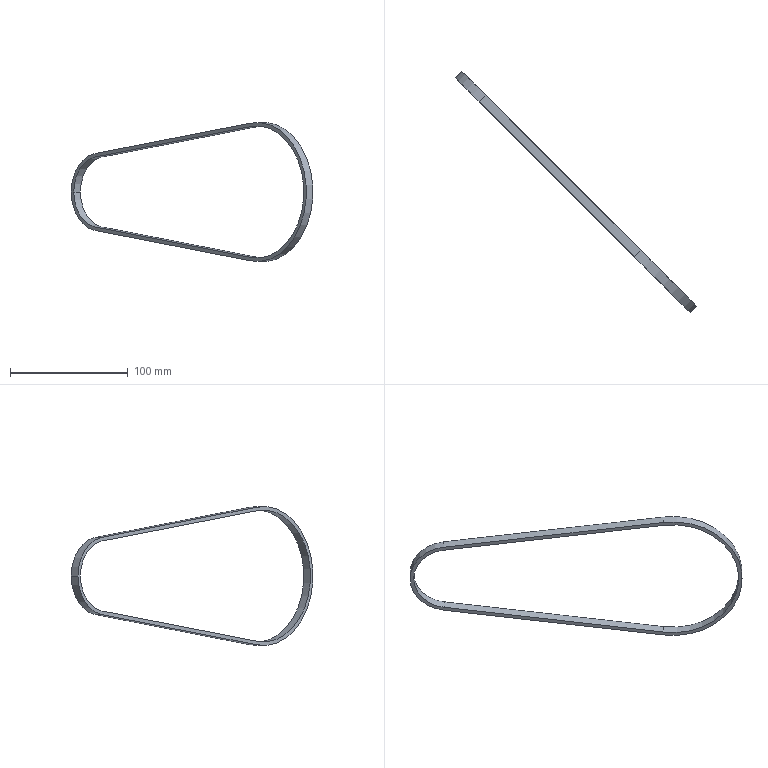Part | SolidWorks | 1 solid | 12 faces | box 205.061 x 205.061 x 118 mm | volume 15916 mm3 | cylinder 6 | plane 6 | commonest cylinder face diameters 60 x2 66 x2 112 x1 118 x1
STEP:
#1=CARTESIAN_POINT('',(92.408,296.784,-1142.11));
#2=VERTEX_POINT('',#1);
#3=CARTESIAN_POINT('',(72.266,316.925,-1109.42));
#4=VERTEX_POINT('',#3);
#5=CARTESIAN_POINT('',(95.601,293.591,-1109.42));
#6=DIRECTION('',(0.7071,0.7071,0.));
#7=DIRECTION('',(-0.7071,0.7071,0.));
#8=AXIS2_PLACEMENT_3D('',#5,#6,#7);
#9=CIRCLE('',#8,33.);
#10=EDGE_CURVE('',#2,#4,#9,.T.);
#11=ORIENTED_EDGE('',*,*,#10,.T.);
#12=CARTESIAN_POINT('',(77.923,322.582,-1109.42));
#13=VERTEX_POINT('',#12);
#14=CARTESIAN_POINT('',(77.923,322.582,-1109.42));
#15=DIRECTION('',(0.7071,0.7071,0.));
#16=VECTOR('',#15,1000.);
#17=LINE('',#14,#16);
#18=EDGE_CURVE('',#4,#13,#17,.T.);
#19=ORIENTED_EDGE('',*,*,#18,.T.);
#20=CARTESIAN_POINT('',(98.065,302.441,-1142.11));
#21=VERTEX_POINT('',#20);
#22=CARTESIAN_POINT('',(101.258,299.248,-1109.42));
#23=DIRECTION('',(-0.7071,-0.7071,0.));
#24=DIRECTION('',(-0.09676,0.09676,0.9906));
#25=AXIS2_PLACEMENT_3D('',#22,#23,#24);
#26=CIRCLE('',#25,33.);
#27=EDGE_CURVE('',#13,#21,#26,.T.);
#28=ORIENTED_EDGE('',*,*,#27,.T.);
#29=CARTESIAN_POINT('',(92.408,296.784,-1142.11));
#30=DIRECTION('',(0.7071,0.7071,0.));
#31=VECTOR('',#30,1000.);
#32=LINE('',#29,#31);
#33=EDGE_CURVE('',#2,#21,#32,.T.);
#34=ORIENTED_EDGE('',*,*,#33,.F.);
#35=EDGE_LOOP('',(#11,#19,#28,#34));
#36=FACE_OUTER_BOUND('',#35,.T.);
#37=CARTESIAN_POINT('',(101.258,299.248,-1109.42));
#38=DIRECTION('',(0.7071,0.7071,0.));
#39=DIRECTION('',(-0.7071,0.7071,0.));
#40=AXIS2_PLACEMENT_3D('',#37,#38,#39);
#41=CYLINDRICAL_SURFACE('',#40,33.);
#42=ADVANCED_FACE('',(#36),#41,.T.);
#43=CARTESIAN_POINT('',(92.698,296.494,-1079.702));
#44=VERTEX_POINT('',#43);
#45=CARTESIAN_POINT('',(74.388,314.804,-1109.42));
#46=VERTEX_POINT('',#45);
#47=CARTESIAN_POINT('',(95.601,293.591,-1109.42));
#48=DIRECTION('',(-0.7071,-0.7071,0.));
#49=DIRECTION('',(-0.09676,0.09676,0.9906));
#50=AXIS2_PLACEMENT_3D('',#47,#48,#49);
#51=CIRCLE('',#50,30.);
#52=EDGE_CURVE('',#44,#46,#51,.T.);
#53=ORIENTED_EDGE('',*,*,#52,.T.);
#54=CARTESIAN_POINT('',(80.044,320.461,-1109.42));
#55=VERTEX_POINT('',#54);
#56=CARTESIAN_POINT('',(80.044,320.461,-1109.42));
#57=DIRECTION('',(0.7071,0.7071,0.));
#58=VECTOR('',#57,1000.);
#59=LINE('',#56,#58);
#60=EDGE_CURVE('',#46,#55,#59,.T.);
#61=ORIENTED_EDGE('',*,*,#60,.T.);
#62=CARTESIAN_POINT('',(98.355,302.15,-1079.702));
#63=VERTEX_POINT('',#62);
#64=CARTESIAN_POINT('',(101.258,299.248,-1109.42));
#65=DIRECTION('',(0.7071,0.7071,0.));
#66=DIRECTION('',(-0.09676,0.09676,-0.9906));
#67=AXIS2_PLACEMENT_3D('',#64,#65,#66);
#68=CIRCLE('',#67,30.);
#69=EDGE_CURVE('',#55,#63,#68,.T.);
#70=ORIENTED_EDGE('',*,*,#69,.T.);
#71=CARTESIAN_POINT('',(92.698,296.494,-1079.702));
#72=DIRECTION('',(0.7071,0.7071,0.));
#73=VECTOR('',#72,1000.);
#74=LINE('',#71,#73);
#75=EDGE_CURVE('',#44,#63,#74,.T.);
#76=ORIENTED_EDGE('',*,*,#75,.F.);
#77=EDGE_LOOP('',(#53,#61,#70,#76));
#78=FACE_OUTER_BOUND('',#77,.T.);
#79=CARTESIAN_POINT('',(101.258,299.248,-1109.42));
#80=DIRECTION('',(0.7071,0.7071,0.));
#81=DIRECTION('',(-0.7071,0.7071,0.));
#82=AXIS2_PLACEMENT_3D('',#79,#80,#81);
#83=CYLINDRICAL_SURFACE('',#82,30.);
#84=ADVANCED_FACE('',(#78),#83,.F.);
#85=ORIENTED_EDGE('',*,*,#60,.F.);
#86=CARTESIAN_POINT('',(92.698,296.494,-1139.138));
#87=VERTEX_POINT('',#86);
#88=CARTESIAN_POINT('',(95.601,293.591,-1109.42));
#89=DIRECTION('',(-0.7071,-0.7071,0.));
#90=DIRECTION('',(-0.09676,0.09676,0.9906));
#91=AXIS2_PLACEMENT_3D('',#88,#89,#90);
#92=CIRCLE('',#91,30.);
#93=EDGE_CURVE('',#46,#87,#92,.T.);
#94=ORIENTED_EDGE('',*,*,#93,.T.);
#95=CARTESIAN_POINT('',(98.355,302.15,-1139.138));
#96=VERTEX_POINT('',#95);
#97=CARTESIAN_POINT('',(98.355,302.15,-1139.138));
#98=DIRECTION('',(-0.7071,-0.7071,0.));
#99=VECTOR('',#98,1000.);
#100=LINE('',#97,#99);
#101=EDGE_CURVE('',#96,#87,#100,.T.);
#102=ORIENTED_EDGE('',*,*,#101,.F.);
#103=CARTESIAN_POINT('',(101.258,299.248,-1109.42));
#104=DIRECTION('',(0.7071,0.7071,0.));
#105=DIRECTION('',(-0.09676,0.09676,-0.9906));
#106=AXIS2_PLACEMENT_3D('',#103,#104,#105);
#107=CIRCLE('',#106,30.);
#108=EDGE_CURVE('',#96,#55,#107,.T.);
#109=ORIENTED_EDGE('',*,*,#108,.T.);
#110=EDGE_LOOP('',(#85,#94,#102,#109));
#111=FACE_OUTER_BOUND('',#110,.T.);
#112=CARTESIAN_POINT('',(101.258,299.248,-1109.42));
#113=DIRECTION('',(0.7071,0.7071,0.));
#114=DIRECTION('',(-0.7071,0.7071,0.));
#115=AXIS2_PLACEMENT_3D('',#112,#113,#114);
#116=CYLINDRICAL_SURFACE('',#115,30.);
#117=ADVANCED_FACE('',(#111),#116,.F.);
#118=ORIENTED_EDGE('',*,*,#101,.T.);
#119=CARTESIAN_POINT('',(224.532,164.659,-1164.893));
#120=VERTEX_POINT('',#119);
#121=CARTESIAN_POINT('',(92.698,296.494,-1139.138));
#122=DIRECTION('',(0.7005,-0.7005,-0.1368));
#123=VECTOR('',#122,1000.);
#124=LINE('',#121,#123);
#125=EDGE_CURVE('',#87,#120,#124,.T.);
#126=ORIENTED_EDGE('',*,*,#125,.T.);
#127=CARTESIAN_POINT('',(230.189,170.316,-1164.893));
#128=VERTEX_POINT('',#127);
#129=CARTESIAN_POINT('',(224.532,164.659,-1164.893));
#130=DIRECTION('',(0.7071,0.7071,0.));
#131=VECTOR('',#130,1000.);
#132=LINE('',#129,#131);
#133=EDGE_CURVE('',#120,#128,#132,.T.);
#134=ORIENTED_EDGE('',*,*,#133,.T.);
#135=CARTESIAN_POINT('',(230.189,170.316,-1164.893));
#136=DIRECTION('',(-0.7005,0.7005,0.1368));
#137=VECTOR('',#136,1000.);
#138=LINE('',#135,#137);
#139=EDGE_CURVE('',#128,#96,#138,.T.);
#140=ORIENTED_EDGE('',*,*,#139,.T.);
#141=EDGE_LOOP('',(#118,#126,#134,#140));
#142=FACE_OUTER_BOUND('',#141,.T.);
#143=CARTESIAN_POINT('',(230.189,170.316,-1164.893));
#144=DIRECTION('',(-0.09676,0.09676,-0.9906));
#145=DIRECTION('',(-0.7005,0.7005,0.1368));
#146=AXIS2_PLACEMENT_3D('',#143,#144,#145);
#147=PLANE('',#146);
#148=ADVANCED_FACE('',(#142),#147,.F.);
#149=ORIENTED_EDGE('',*,*,#133,.F.);
#150=CARTESIAN_POINT('',(224.532,164.659,-1053.947));
#151=VERTEX_POINT('',#150);
#152=CARTESIAN_POINT('',(229.951,159.24,-1109.42));
#153=DIRECTION('',(-0.7071,-0.7071,0.));
#154=DIRECTION('',(-0.09676,0.09676,-0.9906));
#155=AXIS2_PLACEMENT_3D('',#152,#153,#154);
#156=CIRCLE('',#155,56.);
#157=EDGE_CURVE('',#120,#151,#156,.T.);
#158=ORIENTED_EDGE('',*,*,#157,.T.);
#159=CARTESIAN_POINT('',(230.189,170.316,-1053.947));
#160=VERTEX_POINT('',#159);
#161=CARTESIAN_POINT('',(230.189,170.316,-1053.947));
#162=DIRECTION('',(-0.7071,-0.7071,0.));
#163=VECTOR('',#162,1000.);
#164=LINE('',#161,#163);
#165=EDGE_CURVE('',#160,#151,#164,.T.);
#166=ORIENTED_EDGE('',*,*,#165,.F.);
#167=CARTESIAN_POINT('',(235.608,164.897,-1109.42));
#168=DIRECTION('',(0.7071,0.7071,0.));
#169=DIRECTION('',(-0.09676,0.09676,0.9906));
#170=AXIS2_PLACEMENT_3D('',#167,#168,#169);
#171=CIRCLE('',#170,56.);
#172=EDGE_CURVE('',#160,#128,#171,.T.);
#173=ORIENTED_EDGE('',*,*,#172,.T.);
#174=EDGE_LOOP('',(#149,#158,#166,#173));
#175=FACE_OUTER_BOUND('',#174,.T.);
#176=CARTESIAN_POINT('',(235.608,164.897,-1109.42));
#177=DIRECTION('',(0.7071,0.7071,0.));
#178=DIRECTION('',(-0.7071,0.7071,0.));
#179=AXIS2_PLACEMENT_3D('',#176,#177,#178);
#180=CYLINDRICAL_SURFACE('',#179,56.);
#181=ADVANCED_FACE('',(#175),#180,.F.);
#182=ORIENTED_EDGE('',*,*,#125,.F.);
#183=ORIENTED_EDGE('',*,*,#93,.F.);
#184=ORIENTED_EDGE('',*,*,#52,.F.);
#185=CARTESIAN_POINT('',(92.698,296.494,-1079.702));
#186=DIRECTION('',(0.7005,-0.7005,0.1368));
#187=VECTOR('',#186,1000.);
#188=LINE('',#185,#187);
#189=EDGE_CURVE('',#44,#151,#188,.T.);
#190=ORIENTED_EDGE('',*,*,#189,.T.);
#191=ORIENTED_EDGE('',*,*,#157,.F.);
#192=EDGE_LOOP('',(#182,#183,#184,#190,#191));
#193=FACE_BOUND('',#192,.T.);
#194=CARTESIAN_POINT('',(224.242,164.949,-1167.865));
#195=VERTEX_POINT('',#194);
#196=CARTESIAN_POINT('',(224.242,164.949,-1167.865));
#197=DIRECTION('',(-0.7005,0.7005,0.1368));
#198=VECTOR('',#197,1000.);
#199=LINE('',#196,#198);
#200=EDGE_CURVE('',#195,#2,#199,.T.);
#201=ORIENTED_EDGE('',*,*,#200,.F.);
#202=CARTESIAN_POINT('',(224.242,164.949,-1050.975));
#203=VERTEX_POINT('',#202);
#204=CARTESIAN_POINT('',(229.951,159.24,-1109.42));
#205=DIRECTION('',(0.7071,0.7071,0.));
#206=DIRECTION('',(0.09676,-0.09676,-0.9906));
#207=AXIS2_PLACEMENT_3D('',#204,#205,#206);
#208=CIRCLE('',#207,59.);
#209=EDGE_CURVE('',#203,#195,#208,.T.);
#210=ORIENTED_EDGE('',*,*,#209,.F.);
#211=CARTESIAN_POINT('',(92.408,296.784,-1076.73));
#212=VERTEX_POINT('',#211);
#213=CARTESIAN_POINT('',(92.408,296.784,-1076.73));
#214=DIRECTION('',(0.7005,-0.7005,0.1368));
#215=VECTOR('',#214,1000.);
#216=LINE('',#213,#215);
#217=EDGE_CURVE('',#212,#203,#216,.T.);
#218=ORIENTED_EDGE('',*,*,#217,.F.);
#219=CARTESIAN_POINT('',(95.601,293.591,-1109.42));
#220=DIRECTION('',(0.7071,0.7071,0.));
#221=DIRECTION('',(-0.7071,0.7071,0.));
#222=AXIS2_PLACEMENT_3D('',#219,#220,#221);
#223=CIRCLE('',#222,33.);
#224=EDGE_CURVE('',#4,#212,#223,.T.);
#225=ORIENTED_EDGE('',*,*,#224,.F.);
#226=ORIENTED_EDGE('',*,*,#10,.F.);
#227=EDGE_LOOP('',(#201,#210,#218,#225,#226));
#228=FACE_OUTER_BOUND('',#227,.T.);
#229=CARTESIAN_POINT('',(158.47,230.721,-1065.339));
#230=DIRECTION('',(0.7071,0.7071,0.));
#231=DIRECTION('',(0.7005,-0.7005,0.1368));
#232=AXIS2_PLACEMENT_3D('',#229,#230,#231);
#233=PLANE('',#232);
#234=ADVANCED_FACE('',(#193,#228),#233,.F.);
#235=CARTESIAN_POINT('',(98.065,302.441,-1076.73));
#236=VERTEX_POINT('',#235);
#237=CARTESIAN_POINT('',(98.065,302.441,-1076.73));
#238=DIRECTION('',(-0.7071,-0.7071,0.));
#239=VECTOR('',#238,1000.);
#240=LINE('',#237,#239);
#241=EDGE_CURVE('',#236,#212,#240,.T.);
#242=ORIENTED_EDGE('',*,*,#241,.T.);
#243=ORIENTED_EDGE('',*,*,#217,.T.);
#244=CARTESIAN_POINT('',(229.899,170.606,-1050.975));
#245=VERTEX_POINT('',#244);
#246=CARTESIAN_POINT('',(224.242,164.949,-1050.975));
#247=DIRECTION('',(0.7071,0.7071,0.));
#248=VECTOR('',#247,1000.);
#249=LINE('',#246,#248);
#250=EDGE_CURVE('',#203,#245,#249,.T.);
#251=ORIENTED_EDGE('',*,*,#250,.T.);
#252=CARTESIAN_POINT('',(98.065,302.441,-1076.73));
#253=DIRECTION('',(0.7005,-0.7005,0.1368));
#254=VECTOR('',#253,1000.);
#255=LINE('',#252,#254);
#256=EDGE_CURVE('',#236,#245,#255,.T.);
#257=ORIENTED_EDGE('',*,*,#256,.F.);
#258=EDGE_LOOP('',(#242,#243,#251,#257));
#259=FACE_OUTER_BOUND('',#258,.T.);
#260=CARTESIAN_POINT('',(98.065,302.441,-1076.73));
#261=DIRECTION('',(-0.09676,0.09676,0.9906));
#262=DIRECTION('',(0.7005,-0.7005,0.1368));
#263=AXIS2_PLACEMENT_3D('',#260,#261,#262);
#264=PLANE('',#263);
#265=ADVANCED_FACE('',(#259),#264,.T.);
#266=ORIENTED_EDGE('',*,*,#18,.F.);
#267=ORIENTED_EDGE('',*,*,#224,.T.);
#268=ORIENTED_EDGE('',*,*,#241,.F.);
#269=CARTESIAN_POINT('',(101.258,299.248,-1109.42));
#270=DIRECTION('',(-0.7071,-0.7071,0.));
#271=DIRECTION('',(-0.09676,0.09676,0.9906));
#272=AXIS2_PLACEMENT_3D('',#269,#270,#271);
#273=CIRCLE('',#272,33.);
#274=EDGE_CURVE('',#236,#13,#273,.T.);
#275=ORIENTED_EDGE('',*,*,#274,.T.);
#276=EDGE_LOOP('',(#266,#267,#268,#275));
#277=FACE_OUTER_BOUND('',#276,.T.);
#278=CARTESIAN_POINT('',(101.258,299.248,-1109.42));
#279=DIRECTION('',(0.7071,0.7071,0.));
#280=DIRECTION('',(-0.7071,0.7071,0.));
#281=AXIS2_PLACEMENT_3D('',#278,#279,#280);
#282=CYLINDRICAL_SURFACE('',#281,33.);
#283=ADVANCED_FACE('',(#277),#282,.T.);
#284=CARTESIAN_POINT('',(229.899,170.606,-1167.865));
#285=VERTEX_POINT('',#284);
#286=CARTESIAN_POINT('',(229.899,170.606,-1167.865));
#287=DIRECTION('',(-0.7071,-0.7071,0.));
#288=VECTOR('',#287,1000.);
#289=LINE('',#286,#288);
#290=EDGE_CURVE('',#285,#195,#289,.T.);
#291=ORIENTED_EDGE('',*,*,#290,.T.);
#292=ORIENTED_EDGE('',*,*,#200,.T.);
#293=ORIENTED_EDGE('',*,*,#33,.T.);
#294=CARTESIAN_POINT('',(98.065,302.441,-1142.11));
#295=DIRECTION('',(0.7005,-0.7005,-0.1368));
#296=VECTOR('',#295,1000.);
#297=LINE('',#294,#296);
#298=EDGE_CURVE('',#21,#285,#297,.T.);
#299=ORIENTED_EDGE('',*,*,#298,.T.);
#300=EDGE_LOOP('',(#291,#292,#293,#299));
#301=FACE_OUTER_BOUND('',#300,.T.);
#302=CARTESIAN_POINT('',(229.899,170.606,-1167.865));
#303=DIRECTION('',(-0.09676,0.09676,-0.9906));
#304=DIRECTION('',(-0.7005,0.7005,0.1368));
#305=AXIS2_PLACEMENT_3D('',#302,#303,#304);
#306=PLANE('',#305);
#307=ADVANCED_FACE('',(#301),#306,.T.);
#308=ORIENTED_EDGE('',*,*,#250,.F.);
#309=ORIENTED_EDGE('',*,*,#209,.T.);
#310=ORIENTED_EDGE('',*,*,#290,.F.);
#311=CARTESIAN_POINT('',(235.608,164.897,-1109.42));
#312=DIRECTION('',(-0.7071,-0.7071,0.));
#313=DIRECTION('',(-0.09676,0.09676,-0.9906));
#314=AXIS2_PLACEMENT_3D('',#311,#312,#313);
#315=CIRCLE('',#314,59.);
#316=EDGE_CURVE('',#285,#245,#315,.T.);
#317=ORIENTED_EDGE('',*,*,#316,.T.);
#318=EDGE_LOOP('',(#308,#309,#310,#317));
#319=FACE_OUTER_BOUND('',#318,.T.);
#320=CARTESIAN_POINT('',(235.608,164.897,-1109.42));
#321=DIRECTION('',(0.7071,0.7071,0.));
#322=DIRECTION('',(-0.7071,0.7071,0.));
#323=AXIS2_PLACEMENT_3D('',#320,#321,#322);
#324=CYLINDRICAL_SURFACE('',#323,59.);
#325=ADVANCED_FACE('',(#319),#324,.T.);
#326=ORIENTED_EDGE('',*,*,#139,.F.);
#327=ORIENTED_EDGE('',*,*,#172,.F.);
#328=CARTESIAN_POINT('',(98.355,302.15,-1079.702));
#329=DIRECTION('',(0.7005,-0.7005,0.1368));
#330=VECTOR('',#329,1000.);
#331=LINE('',#328,#330);
#332=EDGE_CURVE('',#63,#160,#331,.T.);
#333=ORIENTED_EDGE('',*,*,#332,.F.);
#334=ORIENTED_EDGE('',*,*,#69,.F.);
#335=ORIENTED_EDGE('',*,*,#108,.F.);
#336=EDGE_LOOP('',(#326,#327,#333,#334,#335));
#337=FACE_BOUND('',#336,.T.);
#338=ORIENTED_EDGE('',*,*,#298,.F.);
#339=ORIENTED_EDGE('',*,*,#27,.F.);
#340=ORIENTED_EDGE('',*,*,#274,.F.);
#341=ORIENTED_EDGE('',*,*,#256,.T.);
#342=ORIENTED_EDGE('',*,*,#316,.F.);
#343=EDGE_LOOP('',(#338,#339,#340,#341,#342));
#344=FACE_OUTER_BOUND('',#343,.T.);
#345=CARTESIAN_POINT('',(164.127,236.378,-1065.339));
#346=DIRECTION('',(0.7071,0.7071,0.));
#347=DIRECTION('',(0.7005,-0.7005,0.1368));
#348=AXIS2_PLACEMENT_3D('',#345,#346,#347);
#349=PLANE('',#348);
#350=ADVANCED_FACE('',(#337,#344),#349,.T.);
#351=ORIENTED_EDGE('',*,*,#165,.T.);
#352=ORIENTED_EDGE('',*,*,#189,.F.);
#353=ORIENTED_EDGE('',*,*,#75,.T.);
#354=ORIENTED_EDGE('',*,*,#332,.T.);
#355=EDGE_LOOP('',(#351,#352,#353,#354));
#356=FACE_OUTER_BOUND('',#355,.T.);
#357=CARTESIAN_POINT('',(98.355,302.15,-1079.702));
#358=DIRECTION('',(-0.09676,0.09676,0.9906));
#359=DIRECTION('',(0.7005,-0.7005,0.1368));
#360=AXIS2_PLACEMENT_3D('',#357,#358,#359);
#361=PLANE('',#360);
#362=ADVANCED_FACE('',(#356),#361,.F.);
#363=CLOSED_SHELL('',(#42,#84,#117,#148,#181,#234,#265,#283,#307,#325,#350,#362));
#364=MANIFOLD_SOLID_BREP('',#363);
#365=CARTESIAN_POINT('',(0.,0.,0.));
#366=DIRECTION('',(0.,0.,1.));
#367=DIRECTION('',(1.,0.,0.));
#368=AXIS2_PLACEMENT_3D('',#365,#366,#367);
#369=(LENGTH_UNIT()NAMED_UNIT(*)SI_UNIT(.MILLI.,.METRE.));
#370=UNCERTAINTY_MEASURE_WITH_UNIT(LENGTH_MEASURE(0.00001),#369,'','');
#371=(NAMED_UNIT(*)PLANE_ANGLE_UNIT()SI_UNIT($,.RADIAN.));
#372=(NAMED_UNIT(*)SI_UNIT($,.STERADIAN.)SOLID_ANGLE_UNIT());
#373=(GEOMETRIC_REPRESENTATION_CONTEXT(3)GLOBAL_UNCERTAINTY_ASSIGNED_CONTEXT((#370))GLOBAL_UNIT_ASSIGNED_CONTEXT((#369,#371,#372))REPRESENTATION_CONTEXT('',''));
#374=ADVANCED_BREP_SHAPE_REPRESENTATION('',(#364,#368),#373);